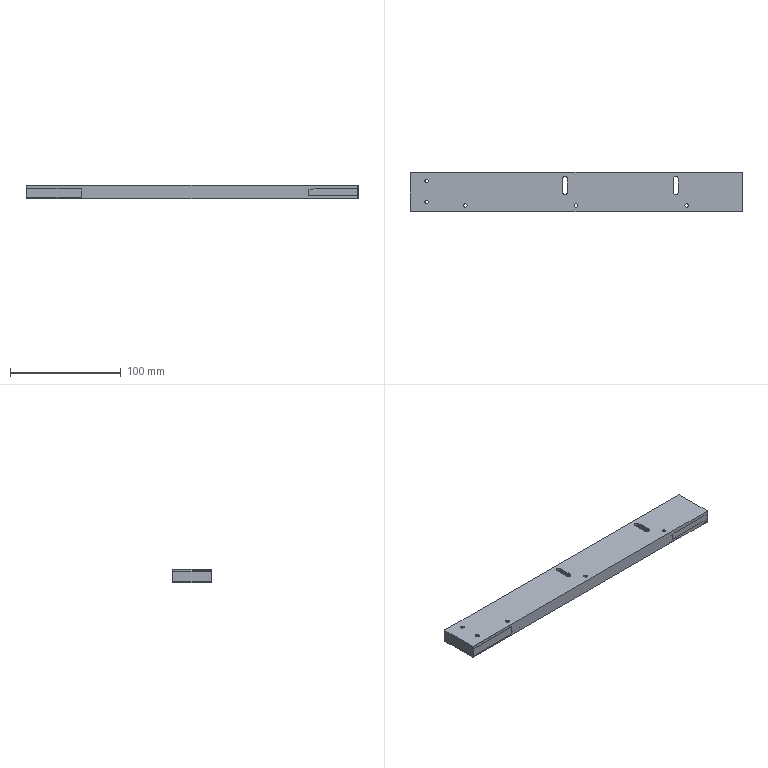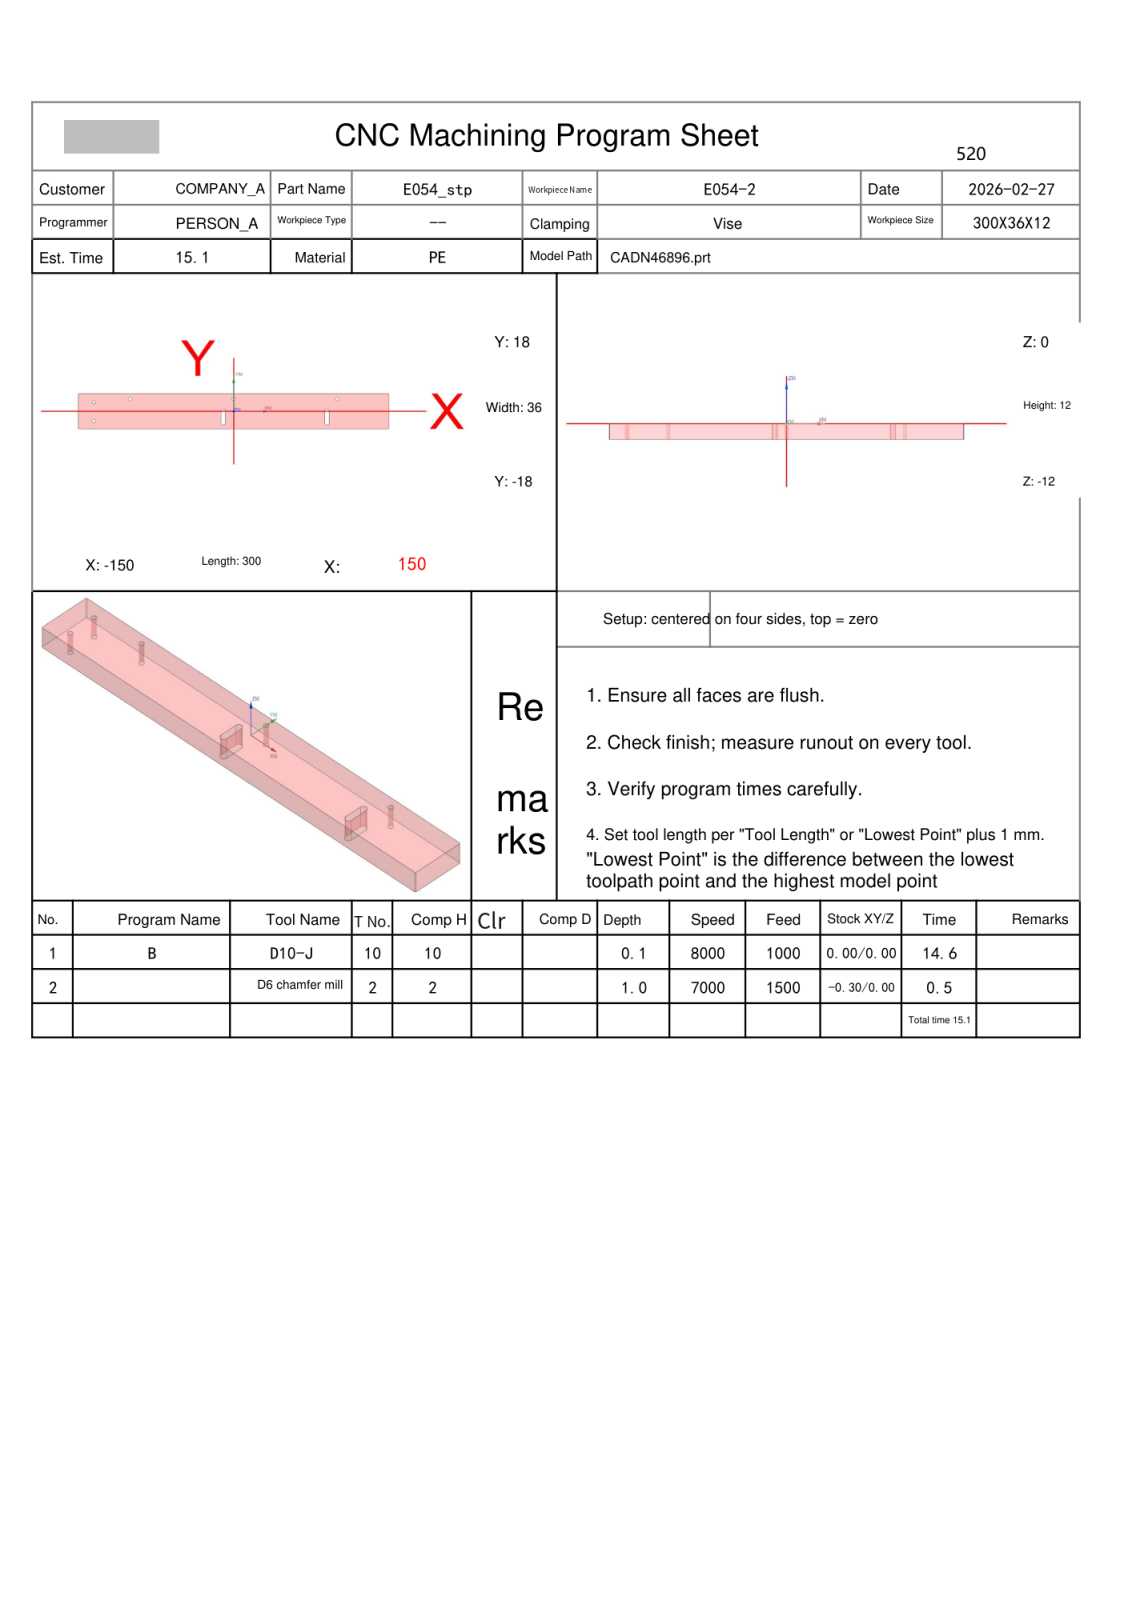NC program | NX | posted by the shop | part box 300 x 36 x 12 mm
Whole program:
%
O0001
(Machine time: 15.47 MIN)
(===Total Tool:2===)
(T10=D10-J  D=10.  R=0.   D-  H10 Z=0.    )
(T2=D6 chamfer mill   D=6.   R=0.   D-  H02 Z=-1.   )
G80 G90 G17 G49 G40
G91 G28 Z0
M01
N1 T10 M06
(D10-J  D=10. R=0. H=10 ce=0.00 di=0.10)
G00 G90 G54 X-167. Y1.111 M03 S8000
G43 H10 Z50.
M08
Z4.02
G01 Z2.02 F1000.
X-155. Y13.111
X-145.111 Y23.
X-135.222
X-155. Y3.222
Y-6.667
X-125.333 Y23.
X-115.444
X-155. Y-16.556
Y-23.
X-151.556
X-105.556 Y23.
X-95.667
X-141.667 Y-23.
X-131.778
X-85.778 Y23.
X-75.889
X-121.889 Y-23.
X-112.
X-66. Y23.
X-56.111
X-102.111 Y-23.
X-92.222
X-46.222 Y23.
X-36.333
X-82.333 Y-23.
X-72.444
X-26.444 Y23.
X-16.556
X-62.556 Y-23.
X-52.667
X-6.667 Y23.
X3.222
X-42.778 Y-23.
X-32.889
X13.111 Y23.
X23.
X-23. Y-23.
X-13.111
X32.889 Y23.
X42.778
X-3.222 Y-23.
X6.667
X52.667 Y23.
X62.556
X16.556 Y-23.
X26.444
X72.444 Y23.
X82.333
X36.333 Y-23.
X46.222
X92.222 Y23.
X102.111
X56.111 Y-23.
X66.
X112. Y23.
X121.889
X75.889 Y-23.
X85.778
X131.778 Y23.
X141.667
X95.667 Y-23.
X105.556
X151.556 Y23.
X155.
Y16.556
X115.444 Y-23.
X125.333
X155. Y6.667
Y-3.222
X135.222 Y-23.
X145.111
X155. Y-13.111
X167. Y-1.111
Z4.02
G00 Z5.5
X-167. Y1.111
Z3.54
G01 Z1.54
X-155. Y13.111
X-145.111 Y23.
X-135.222
X-155. Y3.222
Y-6.667
X-125.333 Y23.
X-115.444
X-155. Y-16.556
Y-23.
X-151.556
X-105.556 Y23.
X-95.667
X-141.667 Y-23.
X-131.778
X-85.778 Y23.
X-75.889
X-121.889 Y-23.
X-112.
X-66. Y23.
X-56.111
X-102.111 Y-23.
X-92.222
X-46.222 Y23.
X-36.333
X-82.333 Y-23.
X-72.444
X-26.444 Y23.
X-16.556
X-62.556 Y-23.
X-52.667
X-6.667 Y23.
X3.222
X-42.778 Y-23.
X-32.889
X13.111 Y23.
X23.
X-23. Y-23.
X-13.111
X32.889 Y23.
X42.778
X-3.222 Y-23.
X6.667
X52.667 Y23.
X62.556
X16.556 Y-23.
X26.444
X72.444 Y23.
X82.333
X36.333 Y-23.
X46.222
X92.222 Y23.
X102.111
X56.111 Y-23.
X66.
X112. Y23.
X121.889
X75.889 Y-23.
X85.778
X131.778 Y23.
X141.667
X95.667 Y-23.
X105.556
X151.556 Y23.
X155.
Y16.556
X115.444 Y-23.
X125.333
X155. Y6.667
Y-3.222
X135.222 Y-23.
X145.111
X155. Y-13.111
X167. Y-1.111
Z3.54
G00 Z5.02
X-167. Y1.111
Z3.06
G01 Z1.06
X-155. Y13.111
X-145.111 Y23.
X-135.222
X-155. Y3.222
Y-6.667
X-125.333 Y23.
X-115.444
X-155. Y-16.556
Y-23.
X-151.556
X-105.556 Y23.
X-95.667
X-141.667 Y-23.
X-131.778
X-85.778 Y23.
X-75.889
X-121.889 Y-23.
X-112.
X-66. Y23.
X-56.111
X-102.111 Y-23.
X-92.222
X-46.222 Y23.
X-36.333
X-82.333 Y-23.
X-72.444
X-26.444 Y23.
X-16.556
X-62.556 Y-23.
X-52.667
X-6.667 Y23.
X3.222
X-42.778 Y-23.
X-32.889
X13.111 Y23.
X23.
X-23. Y-23.
X-13.111
X32.889 Y23.
X42.778
X-3.222 Y-23.
X6.667
X52.667 Y23.
X62.556
X16.556 Y-23.
X26.444
X72.444 Y23.
X82.333
X36.333 Y-23.
X46.222
X92.222 Y23.
X102.111
X56.111 Y-23.
X66.
X112. Y23.
X121.889
X75.889 Y-23.
X85.778
X131.778 Y23.
X141.667
X95.667 Y-23.
X105.556
X151.556 Y23.
X155.
Y16.556
X115.444 Y-23.
X125.333
X155. Y6.667
Y-3.222
X135.222 Y-23.
X145.111
X155. Y-13.111
X167. Y-1.111
Z3.06
G00 Z4.54
X-167. Y1.111
Z2.58
G01 Z.58
X-155. Y13.111
X-145.111 Y23.
X-135.222
X-155. Y3.222
Y-6.667
X-125.333 Y23.
X-115.444
X-155. Y-16.556
Y-23.
X-151.556
X-105.556 Y23.
X-95.667
X-141.667 Y-23.
X-131.778
X-85.778 Y23.
X-75.889
X-121.889 Y-23.
X-112.
X-66. Y23.
X-56.111
X-102.111 Y-23.
X-92.222
X-46.222 Y23.
X-36.333
X-82.333 Y-23.
X-72.444
X-26.444 Y23.
X-16.556
X-62.556 Y-23.
X-52.667
X-6.667 Y23.
X3.222
X-42.778 Y-23.
X-32.889
X13.111 Y23.
X23.
X-23. Y-23.
X-13.111
X32.889 Y23.
X42.778
X-3.222 Y-23.
X6.667
X52.667 Y23.
X62.556
X16.556 Y-23.
X26.444
X72.444 Y23.
X82.333
X36.333 Y-23.
X46.222
X92.222 Y23.
X102.111
X56.111 Y-23.
X66.
X112. Y23.
X121.889
X75.889 Y-23.
X85.778
X131.778 Y23.
X141.667
X95.667 Y-23.
X105.556
X151.556 Y23.
X155.
Y16.556
X115.444 Y-23.
X125.333
X155. Y6.667
Y-3.222
X135.222 Y-23.
X145.111
X155. Y-13.111
X167. Y-1.111
Z2.58
G00 Z4.06
X-167. Y1.111
Z2.1
G01 Z.1
X-155. Y13.111
X-145.111 Y23.
X-135.222
X-155. Y3.222
Y-6.667
X-125.333 Y23.
X-115.444
X-155. Y-16.556
Y-23.
X-151.556
X-105.556 Y23.
X-95.667
X-141.667 Y-23.
X-131.778
X-85.778 Y23.
X-75.889
X-121.889 Y-23.
X-112.
X-66. Y23.
X-56.111
X-102.111 Y-23.
X-92.222
X-46.222 Y23.
X-36.333
X-82.333 Y-23.
X-72.444
X-26.444 Y23.
X-16.556
X-62.556 Y-23.
X-52.667
X-6.667 Y23.
X3.222
X-42.778 Y-23.
X-32.889
X13.111 Y23.
X23.
X-23. Y-23.
X-13.111
X32.889 Y23.
X42.778
X-3.222 Y-23.
X6.667
X52.667 Y23.
X62.556
X16.556 Y-23.
X26.444
X72.444 Y23.
X82.333
X36.333 Y-23.
X46.222
X92.222 Y23.
X102.111
X56.111 Y-23.
X66.
X112. Y23.
X121.889
X75.889 Y-23.
X85.778
X131.778 Y23.
X141.667
X95.667 Y-23.
X105.556
X151.556 Y23.
X155.
Y16.556
X115.444 Y-23.
X125.333
X155. Y6.667
Y-3.222
X135.222 Y-23.
X145.111
X155. Y-13.111
X167. Y-1.111
Z2.1
G00 Z50.
G00 G90 X-167. Y1.111 M03 S8000
Z50.
Z2.
G01 Z0.0 F1000.
X-155. Y13.111
X-145.111 Y23.
X-135.222
X-155. Y3.222
Y-6.667
X-125.333 Y23.
X-115.444
X-155. Y-16.556
Y-23.
X-151.556
X-105.556 Y23.
X-95.667
X-141.667 Y-23.
X-131.778
X-85.778 Y23.
X-75.889
X-121.889 Y-23.
X-112.
X-66. Y23.
X-56.111
X-102.111 Y-23.
X-92.222
X-46.222 Y23.
X-36.333
X-82.333 Y-23.
X-72.444
X-26.444 Y23.
X-16.556
X-62.556 Y-23.
X-52.667
X-6.667 Y23.
X3.222
X-42.778 Y-23.
X-32.889
X13.111 Y23.
X23.
X-23. Y-23.
X-13.111
X32.889 Y23.
X42.778
X-3.222 Y-23.
X6.667
X52.667 Y23.
X62.556
X16.556 Y-23.
X26.444
X72.444 Y23.
X82.333
X36.333 Y-23.
X46.222
X92.222 Y23.
X102.111
X56.111 Y-23.
X66.
X112. Y23.
X121.889
X75.889 Y-23.
X85.778
X131.778 Y23.
X141.667
X95.667 Y-23.
X105.556
X151.556 Y23.
X155.
Y16.556
X115.444 Y-23.
X125.333
X155. Y6.667
Y-3.222
X135.222 Y-23.
X145.111
X155. Y-13.111
X167. Y-1.111
Z2.
G00 Z50.
G91 G28 Z0.0
M05
M09
G91 G28 Z0.0
M01
N2 T02 M06
(D6 chamfer mill  D=6. R=0. H=02 ce=-0.30 di=0.00)
G00 G90 G54 X141.791 Y18.7 M03 S7000
G43 H02 Z50.
M08
Z2.5
G01 X149.453 Z-.289 F1500.
X149.66 Y18.662 Z-.365
X149.855 Y18.581 Z-.442
X150.028 Y18.462 Z-.519
X150.462 Y18.028 Z-.742
X150.581 Y17.855 Z-.819
X150.662 Y17.66 Z-.895
X150.7 Y17.453 Z-.972
Y17.376 Z-1.
Y-17.376
G02 X150.407 Y-18.083 I-1. J0.0
G01 X150.083 Y-18.407
G02 X149.376 Y-18.7 I-.707 J.707
G01 X-149.376
G02 X-150.083 Y-18.407 I0.0 J1.
G01 X-150.407 Y-18.083
G02 X-150.7 Y-17.376 I.707 J.707
G01 Y17.376
G02 X-150.407 Y18.083 I1. J0.0
G01 X-150.083 Y18.407
G02 X-149.376 Y18.7 I.707 J-.707
G01 X149.376
G02 X150.083 Y18.407 I0.0 J-1.
G01 X150.407 Y18.083
G02 X150.7 Y17.376 I-.707 J-.707
G01 Y16.876
Z1.5
G00 Z50.
M05
M09
G91 G28 Z0.0
G91 G28 Y0.0
M30
%